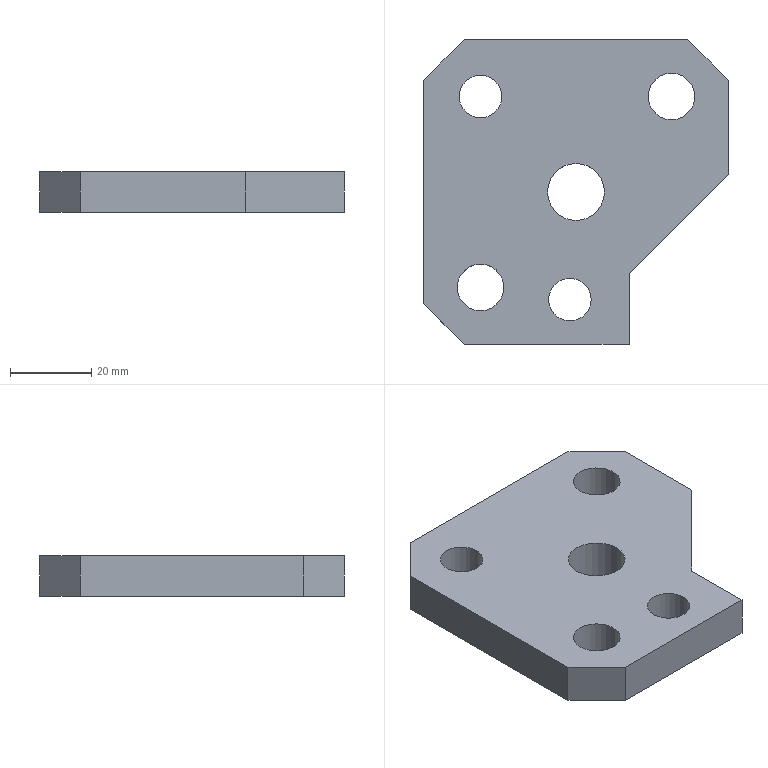Part | NX | features 23 2 | 1 solid | 16 faces | box 75 x 75 x 10 mm | volume 42165 mm3 | plane 11 | cylinder 5 | commonest cylinder face diameters 10.5 x2 11.509 x2 14 x1
STEP:
#1=CARTESIAN_POINT('',(80.279,385.45,-43.5));
#2=VERTEX_POINT('',#1);
#3=CARTESIAN_POINT('',(85.529,385.45,-43.5));
#4=DIRECTION('',(0.,0.,-1.));
#5=DIRECTION('',(-1.,0.,0.));
#6=AXIS2_PLACEMENT_3D('',#3,#4,#5);
#7=CIRCLE('',#6,5.25);
#8=EDGE_CURVE('',#2,#2,#7,.T.);
#9=ORIENTED_EDGE('',*,*,#8,.T.);
#10=EDGE_LOOP('',(#9));
#11=FACE_BOUND('',#10,.T.);
#12=CARTESIAN_POINT('',(80.279,385.45,-33.5));
#13=VERTEX_POINT('',#12);
#14=CARTESIAN_POINT('',(85.529,385.45,-33.5));
#15=DIRECTION('',(0.,0.,-1.));
#16=DIRECTION('',(-1.,0.,0.));
#17=AXIS2_PLACEMENT_3D('',#14,#15,#16);
#18=CIRCLE('',#17,5.25);
#19=EDGE_CURVE('',#13,#13,#18,.T.);
#20=ORIENTED_EDGE('',*,*,#19,.F.);
#21=EDGE_LOOP('',(#20));
#22=FACE_BOUND('',#21,.T.);
#23=CARTESIAN_POINT('',(85.529,385.45,-33.5));
#24=DIRECTION('',(0.,0.,-1.));
#25=DIRECTION('',(0.,-1.,0.));
#26=AXIS2_PLACEMENT_3D('',#23,#24,#25);
#27=CYLINDRICAL_SURFACE('',#26,5.25);
#28=ADVANCED_FACE('',(#11,#22),#27,.F.);
#29=CARTESIAN_POINT('',(80.029,411.95,-33.5));
#30=VERTEX_POINT('',#29);
#31=CARTESIAN_POINT('',(87.029,411.95,-33.5));
#32=DIRECTION('',(0.,0.,1.));
#33=DIRECTION('',(-1.,0.,0.));
#34=AXIS2_PLACEMENT_3D('',#31,#32,#33);
#35=CIRCLE('',#34,7.);
#36=EDGE_CURVE('',#30,#30,#35,.T.);
#37=ORIENTED_EDGE('',*,*,#36,.T.);
#38=EDGE_LOOP('',(#37));
#39=FACE_BOUND('',#38,.T.);
#40=CARTESIAN_POINT('',(80.029,411.95,-43.5));
#41=VERTEX_POINT('',#40);
#42=CARTESIAN_POINT('',(87.029,411.95,-43.5));
#43=DIRECTION('',(0.,0.,1.));
#44=DIRECTION('',(-1.,0.,0.));
#45=AXIS2_PLACEMENT_3D('',#42,#43,#44);
#46=CIRCLE('',#45,7.);
#47=EDGE_CURVE('',#41,#41,#46,.T.);
#48=ORIENTED_EDGE('',*,*,#47,.F.);
#49=EDGE_LOOP('',(#48));
#50=FACE_BOUND('',#49,.T.);
#51=CARTESIAN_POINT('',(87.029,411.95,-33.5));
#52=DIRECTION('',(0.,0.,1.));
#53=DIRECTION('',(0.,1.,0.));
#54=AXIS2_PLACEMENT_3D('',#51,#52,#53);
#55=CYLINDRICAL_SURFACE('',#54,7.);
#56=ADVANCED_FACE('',(#39,#50),#55,.F.);
#57=CARTESIAN_POINT('',(49.529,384.45,-33.5));
#58=VERTEX_POINT('',#57);
#59=CARTESIAN_POINT('',(59.529,374.45,-33.5));
#60=VERTEX_POINT('',#59);
#61=CARTESIAN_POINT('',(55.537,378.441,-33.5));
#62=DIRECTION('',(0.7071,-0.7071,0.));
#63=VECTOR('',#62,1000.);
#64=LINE('',#61,#63);
#65=EDGE_CURVE('',#58,#60,#64,.T.);
#66=ORIENTED_EDGE('',*,*,#65,.F.);
#67=CARTESIAN_POINT('',(49.529,384.45,-43.5));
#68=VERTEX_POINT('',#67);
#69=CARTESIAN_POINT('',(49.529,384.45,-33.5));
#70=DIRECTION('',(0.,0.,1.));
#71=VECTOR('',#70,1000.);
#72=LINE('',#69,#71);
#73=EDGE_CURVE('',#68,#58,#72,.T.);
#74=ORIENTED_EDGE('',*,*,#73,.F.);
#75=CARTESIAN_POINT('',(59.529,374.45,-43.5));
#76=VERTEX_POINT('',#75);
#77=CARTESIAN_POINT('',(54.529,379.45,-43.5));
#78=DIRECTION('',(-0.7071,0.7071,0.));
#79=VECTOR('',#78,1000.);
#80=LINE('',#77,#79);
#81=EDGE_CURVE('',#76,#68,#80,.T.);
#82=ORIENTED_EDGE('',*,*,#81,.F.);
#83=CARTESIAN_POINT('',(59.529,374.45,-33.5));
#84=DIRECTION('',(0.,0.,-1.));
#85=VECTOR('',#84,1000.);
#86=LINE('',#83,#85);
#87=EDGE_CURVE('',#60,#76,#86,.T.);
#88=ORIENTED_EDGE('',*,*,#87,.F.);
#89=EDGE_LOOP('',(#66,#74,#82,#88));
#90=FACE_BOUND('',#89,.T.);
#91=CARTESIAN_POINT('',(54.529,379.45,-23.5));
#92=DIRECTION('',(0.7071,0.7071,0.));
#93=DIRECTION('',(0.,0.,1.));
#94=AXIS2_PLACEMENT_3D('',#91,#92,#93);
#95=PLANE('',#94);
#96=ADVANCED_FACE('',(#90),#95,.F.);
#97=CARTESIAN_POINT('',(49.529,439.45,-33.5));
#98=VERTEX_POINT('',#97);
#99=CARTESIAN_POINT('',(49.529,411.95,-33.5));
#100=DIRECTION('',(0.,-1.,0.));
#101=VECTOR('',#100,1000.);
#102=LINE('',#99,#101);
#103=EDGE_CURVE('',#98,#58,#102,.T.);
#104=ORIENTED_EDGE('',*,*,#103,.F.);
#105=CARTESIAN_POINT('',(49.529,439.45,-43.5));
#106=VERTEX_POINT('',#105);
#107=CARTESIAN_POINT('',(49.529,439.45,-33.5));
#108=DIRECTION('',(0.,0.,-1.));
#109=VECTOR('',#108,1000.);
#110=LINE('',#107,#109);
#111=EDGE_CURVE('',#98,#106,#110,.T.);
#112=ORIENTED_EDGE('',*,*,#111,.T.);
#113=CARTESIAN_POINT('',(49.529,444.376,-43.5));
#114=DIRECTION('',(0.,-1.,0.));
#115=VECTOR('',#114,1000.);
#116=LINE('',#113,#115);
#117=EDGE_CURVE('',#106,#68,#116,.T.);
#118=ORIENTED_EDGE('',*,*,#117,.T.);
#119=ORIENTED_EDGE('',*,*,#73,.T.);
#120=EDGE_LOOP('',(#104,#112,#118,#119));
#121=FACE_BOUND('',#120,.T.);
#122=CARTESIAN_POINT('',(49.529,411.95,-33.5));
#123=DIRECTION('',(1.,0.,0.));
#124=DIRECTION('',(0.,-1.,0.));
#125=AXIS2_PLACEMENT_3D('',#122,#123,#124);
#126=PLANE('',#125);
#127=ADVANCED_FACE('',(#121),#126,.F.);
#128=CARTESIAN_POINT('',(59.529,449.45,-33.5));
#129=VERTEX_POINT('',#128);
#130=CARTESIAN_POINT('',(87.964,477.885,-33.5));
#131=DIRECTION('',(-0.7071,-0.7071,0.));
#132=VECTOR('',#131,1000.);
#133=LINE('',#130,#132);
#134=EDGE_CURVE('',#129,#98,#133,.T.);
#135=ORIENTED_EDGE('',*,*,#134,.F.);
#136=CARTESIAN_POINT('',(59.529,449.45,-43.5));
#137=VERTEX_POINT('',#136);
#138=CARTESIAN_POINT('',(59.529,449.45,-33.5));
#139=DIRECTION('',(0.,0.,1.));
#140=VECTOR('',#139,1000.);
#141=LINE('',#138,#140);
#142=EDGE_CURVE('',#137,#129,#141,.T.);
#143=ORIENTED_EDGE('',*,*,#142,.F.);
#144=CARTESIAN_POINT('',(54.529,444.45,-43.5));
#145=DIRECTION('',(0.7071,0.7071,0.));
#146=VECTOR('',#145,1000.);
#147=LINE('',#144,#146);
#148=EDGE_CURVE('',#106,#137,#147,.T.);
#149=ORIENTED_EDGE('',*,*,#148,.F.);
#150=ORIENTED_EDGE('',*,*,#111,.F.);
#151=EDGE_LOOP('',(#135,#143,#149,#150));
#152=FACE_BOUND('',#151,.T.);
#153=CARTESIAN_POINT('',(54.529,444.45,-23.5));
#154=DIRECTION('',(0.7071,-0.7071,0.));
#155=DIRECTION('',(0.,0.,1.));
#156=AXIS2_PLACEMENT_3D('',#153,#154,#155);
#157=PLANE('',#156);
#158=ADVANCED_FACE('',(#152),#157,.F.);
#159=CARTESIAN_POINT('',(114.529,449.45,-33.5));
#160=VERTEX_POINT('',#159);
#161=CARTESIAN_POINT('',(87.029,449.45,-33.5));
#162=DIRECTION('',(-1.,0.,0.));
#163=VECTOR('',#162,1000.);
#164=LINE('',#161,#163);
#165=EDGE_CURVE('',#160,#129,#164,.T.);
#166=ORIENTED_EDGE('',*,*,#165,.F.);
#167=CARTESIAN_POINT('',(114.529,449.45,-43.5));
#168=VERTEX_POINT('',#167);
#169=CARTESIAN_POINT('',(114.529,449.45,-33.5));
#170=DIRECTION('',(0.,0.,-1.));
#171=VECTOR('',#170,1000.);
#172=LINE('',#169,#171);
#173=EDGE_CURVE('',#160,#168,#172,.T.);
#174=ORIENTED_EDGE('',*,*,#173,.T.);
#175=CARTESIAN_POINT('',(121.472,449.45,-43.5));
#176=DIRECTION('',(-1.,0.,0.));
#177=VECTOR('',#176,1000.);
#178=LINE('',#175,#177);
#179=EDGE_CURVE('',#168,#137,#178,.T.);
#180=ORIENTED_EDGE('',*,*,#179,.T.);
#181=ORIENTED_EDGE('',*,*,#142,.T.);
#182=EDGE_LOOP('',(#166,#174,#180,#181));
#183=FACE_BOUND('',#182,.T.);
#184=CARTESIAN_POINT('',(87.029,449.45,-33.5));
#185=DIRECTION('',(0.,-1.,0.));
#186=DIRECTION('',(-1.,0.,0.));
#187=AXIS2_PLACEMENT_3D('',#184,#185,#186);
#188=PLANE('',#187);
#189=ADVANCED_FACE('',(#183),#188,.F.);
#190=CARTESIAN_POINT('',(124.529,439.45,-33.5));
#191=VERTEX_POINT('',#190);
#192=CARTESIAN_POINT('',(120.537,443.441,-33.5));
#193=DIRECTION('',(-0.7071,0.7071,0.));
#194=VECTOR('',#193,1000.);
#195=LINE('',#192,#194);
#196=EDGE_CURVE('',#191,#160,#195,.T.);
#197=ORIENTED_EDGE('',*,*,#196,.F.);
#198=CARTESIAN_POINT('',(124.529,439.45,-43.5));
#199=VERTEX_POINT('',#198);
#200=CARTESIAN_POINT('',(124.529,439.45,-33.5));
#201=DIRECTION('',(0.,0.,1.));
#202=VECTOR('',#201,1000.);
#203=LINE('',#200,#202);
#204=EDGE_CURVE('',#199,#191,#203,.T.);
#205=ORIENTED_EDGE('',*,*,#204,.F.);
#206=CARTESIAN_POINT('',(124.529,439.45,-43.5));
#207=DIRECTION('',(0.7071,-0.7071,0.));
#208=VECTOR('',#207,1000.);
#209=LINE('',#206,#208);
#210=EDGE_CURVE('',#168,#199,#209,.T.);
#211=ORIENTED_EDGE('',*,*,#210,.F.);
#212=ORIENTED_EDGE('',*,*,#173,.F.);
#213=EDGE_LOOP('',(#197,#205,#211,#212));
#214=FACE_BOUND('',#213,.T.);
#215=CARTESIAN_POINT('',(124.529,439.45,-23.5));
#216=DIRECTION('',(-0.7071,-0.7071,0.));
#217=DIRECTION('',(0.,0.,1.));
#218=AXIS2_PLACEMENT_3D('',#215,#216,#217);
#219=PLANE('',#218);
#220=ADVANCED_FACE('',(#214),#219,.F.);
#221=CARTESIAN_POINT('',(124.529,416.278,-43.5));
#222=VERTEX_POINT('',#221);
#223=CARTESIAN_POINT('',(124.529,444.376,-43.5));
#224=DIRECTION('',(0.,1.,0.));
#225=VECTOR('',#224,1000.);
#226=LINE('',#223,#225);
#227=EDGE_CURVE('',#222,#199,#226,.T.);
#228=ORIENTED_EDGE('',*,*,#227,.T.);
#229=ORIENTED_EDGE('',*,*,#204,.T.);
#230=CARTESIAN_POINT('',(124.529,416.278,-33.5));
#231=VERTEX_POINT('',#230);
#232=CARTESIAN_POINT('',(124.529,411.95,-33.5));
#233=DIRECTION('',(0.,1.,0.));
#234=VECTOR('',#233,1000.);
#235=LINE('',#232,#234);
#236=EDGE_CURVE('',#231,#191,#235,.T.);
#237=ORIENTED_EDGE('',*,*,#236,.F.);
#238=CARTESIAN_POINT('',(124.529,416.278,-33.5));
#239=DIRECTION('',(0.,0.,-1.));
#240=VECTOR('',#239,1000.);
#241=LINE('',#238,#240);
#242=EDGE_CURVE('',#231,#222,#241,.T.);
#243=ORIENTED_EDGE('',*,*,#242,.T.);
#244=EDGE_LOOP('',(#228,#229,#237,#243));
#245=FACE_BOUND('',#244,.T.);
#246=CARTESIAN_POINT('',(124.529,411.95,-33.5));
#247=DIRECTION('',(-1.,0.,0.));
#248=DIRECTION('',(0.,1.,0.));
#249=AXIS2_PLACEMENT_3D('',#246,#247,#248);
#250=PLANE('',#249);
#251=ADVANCED_FACE('',(#245),#250,.F.);
#252=CARTESIAN_POINT('',(100.109,391.859,-33.5));
#253=VERTEX_POINT('',#252);
#254=CARTESIAN_POINT('',(137.049,428.799,-33.5));
#255=DIRECTION('',(0.7071,0.7071,0.));
#256=VECTOR('',#255,1000.);
#257=LINE('',#254,#256);
#258=EDGE_CURVE('',#253,#231,#257,.T.);
#259=ORIENTED_EDGE('',*,*,#258,.F.);
#260=CARTESIAN_POINT('',(100.109,391.859,-43.5));
#261=VERTEX_POINT('',#260);
#262=CARTESIAN_POINT('',(100.109,391.859,-33.5));
#263=DIRECTION('',(0.,0.,-1.));
#264=VECTOR('',#263,1000.);
#265=LINE('',#262,#264);
#266=EDGE_CURVE('',#253,#261,#265,.T.);
#267=ORIENTED_EDGE('',*,*,#266,.T.);
#268=CARTESIAN_POINT('',(123.114,414.864,-43.5));
#269=DIRECTION('',(-0.7071,-0.7071,0.));
#270=VECTOR('',#269,1000.);
#271=LINE('',#268,#270);
#272=EDGE_CURVE('',#222,#261,#271,.T.);
#273=ORIENTED_EDGE('',*,*,#272,.F.);
#274=ORIENTED_EDGE('',*,*,#242,.F.);
#275=EDGE_LOOP('',(#259,#267,#273,#274));
#276=FACE_BOUND('',#275,.T.);
#277=CARTESIAN_POINT('',(123.114,414.864,-33.5));
#278=DIRECTION('',(-0.7071,0.7071,0.));
#279=DIRECTION('',(0.,0.,-1.));
#280=AXIS2_PLACEMENT_3D('',#277,#278,#279);
#281=PLANE('',#280);
#282=ADVANCED_FACE('',(#276),#281,.F.);
#283=CARTESIAN_POINT('',(100.109,374.45,-43.5));
#284=VERTEX_POINT('',#283);
#285=CARTESIAN_POINT('',(100.109,444.376,-43.5));
#286=DIRECTION('',(0.,-1.,0.));
#287=VECTOR('',#286,1000.);
#288=LINE('',#285,#287);
#289=EDGE_CURVE('',#261,#284,#288,.T.);
#290=ORIENTED_EDGE('',*,*,#289,.F.);
#291=ORIENTED_EDGE('',*,*,#266,.F.);
#292=CARTESIAN_POINT('',(100.109,374.45,-33.5));
#293=VERTEX_POINT('',#292);
#294=CARTESIAN_POINT('',(100.109,392.723,-33.5));
#295=DIRECTION('',(0.,1.,0.));
#296=VECTOR('',#295,1000.);
#297=LINE('',#294,#296);
#298=EDGE_CURVE('',#293,#253,#297,.T.);
#299=ORIENTED_EDGE('',*,*,#298,.F.);
#300=CARTESIAN_POINT('',(100.109,374.45,-8.5));
#301=DIRECTION('',(0.,0.,1.));
#302=VECTOR('',#301,1000.);
#303=LINE('',#300,#302);
#304=EDGE_CURVE('',#284,#293,#303,.T.);
#305=ORIENTED_EDGE('',*,*,#304,.F.);
#306=EDGE_LOOP('',(#290,#291,#299,#305));
#307=FACE_BOUND('',#306,.T.);
#308=CARTESIAN_POINT('',(100.109,392.723,-8.5));
#309=DIRECTION('',(-1.,0.,0.));
#310=DIRECTION('',(0.,0.,1.));
#311=AXIS2_PLACEMENT_3D('',#308,#309,#310);
#312=PLANE('',#311);
#313=ADVANCED_FACE('',(#307),#312,.F.);
#314=CARTESIAN_POINT('',(121.472,374.45,-43.5));
#315=DIRECTION('',(1.,0.,0.));
#316=VECTOR('',#315,1000.);
#317=LINE('',#314,#316);
#318=EDGE_CURVE('',#76,#284,#317,.T.);
#319=ORIENTED_EDGE('',*,*,#318,.T.);
#320=ORIENTED_EDGE('',*,*,#304,.T.);
#321=CARTESIAN_POINT('',(87.029,374.45,-33.5));
#322=DIRECTION('',(1.,0.,0.));
#323=VECTOR('',#322,1000.);
#324=LINE('',#321,#323);
#325=EDGE_CURVE('',#60,#293,#324,.T.);
#326=ORIENTED_EDGE('',*,*,#325,.F.);
#327=ORIENTED_EDGE('',*,*,#87,.T.);
#328=EDGE_LOOP('',(#319,#320,#326,#327));
#329=FACE_BOUND('',#328,.T.);
#330=CARTESIAN_POINT('',(87.029,374.45,-33.5));
#331=DIRECTION('',(0.,1.,0.));
#332=DIRECTION('',(1.,0.,0.));
#333=AXIS2_PLACEMENT_3D('',#330,#331,#332);
#334=PLANE('',#333);
#335=ADVANCED_FACE('',(#329),#334,.F.);
#336=CARTESIAN_POINT('',(110.529,429.695,-43.5));
#337=VERTEX_POINT('',#336);
#338=CARTESIAN_POINT('',(110.529,435.45,-43.5));
#339=DIRECTION('',(0.,0.,-1.));
#340=DIRECTION('',(0.,-1.,0.));
#341=AXIS2_PLACEMENT_3D('',#338,#339,#340);
#342=CIRCLE('',#341,5.755);
#343=EDGE_CURVE('',#337,#337,#342,.T.);
#344=ORIENTED_EDGE('',*,*,#343,.T.);
#345=EDGE_LOOP('',(#344));
#346=FACE_BOUND('',#345,.T.);
#347=CARTESIAN_POINT('',(110.529,429.695,-33.5));
#348=VERTEX_POINT('',#347);
#349=CARTESIAN_POINT('',(110.529,435.45,-33.5));
#350=DIRECTION('',(0.,0.,-1.));
#351=DIRECTION('',(0.,-1.,0.));
#352=AXIS2_PLACEMENT_3D('',#349,#350,#351);
#353=CIRCLE('',#352,5.755);
#354=EDGE_CURVE('',#348,#348,#353,.T.);
#355=ORIENTED_EDGE('',*,*,#354,.F.);
#356=EDGE_LOOP('',(#355));
#357=FACE_BOUND('',#356,.T.);
#358=CARTESIAN_POINT('',(110.529,435.45,-33.5));
#359=DIRECTION('',(0.,0.,-1.));
#360=DIRECTION('',(0.,-1.,0.));
#361=AXIS2_PLACEMENT_3D('',#358,#359,#360);
#362=CYLINDRICAL_SURFACE('',#361,5.755);
#363=ADVANCED_FACE('',(#346,#357),#362,.F.);
#364=CARTESIAN_POINT('',(63.529,430.2,-43.5));
#365=VERTEX_POINT('',#364);
#366=CARTESIAN_POINT('',(63.529,435.45,-43.5));
#367=DIRECTION('',(0.,0.,-1.));
#368=DIRECTION('',(0.,-1.,0.));
#369=AXIS2_PLACEMENT_3D('',#366,#367,#368);
#370=CIRCLE('',#369,5.25);
#371=EDGE_CURVE('',#365,#365,#370,.T.);
#372=ORIENTED_EDGE('',*,*,#371,.T.);
#373=EDGE_LOOP('',(#372));
#374=FACE_BOUND('',#373,.T.);
#375=CARTESIAN_POINT('',(63.529,430.2,-33.5));
#376=VERTEX_POINT('',#375);
#377=CARTESIAN_POINT('',(63.529,435.45,-33.5));
#378=DIRECTION('',(0.,0.,-1.));
#379=DIRECTION('',(0.,-1.,0.));
#380=AXIS2_PLACEMENT_3D('',#377,#378,#379);
#381=CIRCLE('',#380,5.25);
#382=EDGE_CURVE('',#376,#376,#381,.T.);
#383=ORIENTED_EDGE('',*,*,#382,.F.);
#384=EDGE_LOOP('',(#383));
#385=FACE_BOUND('',#384,.T.);
#386=CARTESIAN_POINT('',(63.529,435.45,-33.5));
#387=DIRECTION('',(0.,0.,-1.));
#388=DIRECTION('',(0.,-1.,0.));
#389=AXIS2_PLACEMENT_3D('',#386,#387,#388);
#390=CYLINDRICAL_SURFACE('',#389,5.25);
#391=ADVANCED_FACE('',(#374,#385),#390,.F.);
#392=CARTESIAN_POINT('',(63.529,382.695,-43.5));
#393=VERTEX_POINT('',#392);
#394=CARTESIAN_POINT('',(63.529,388.45,-43.5));
#395=DIRECTION('',(0.,0.,-1.));
#396=DIRECTION('',(0.,-1.,0.));
#397=AXIS2_PLACEMENT_3D('',#394,#395,#396);
#398=CIRCLE('',#397,5.755);
#399=EDGE_CURVE('',#393,#393,#398,.T.);
#400=ORIENTED_EDGE('',*,*,#399,.T.);
#401=EDGE_LOOP('',(#400));
#402=FACE_BOUND('',#401,.T.);
#403=CARTESIAN_POINT('',(63.529,382.695,-33.5));
#404=VERTEX_POINT('',#403);
#405=CARTESIAN_POINT('',(63.529,388.45,-33.5));
#406=DIRECTION('',(0.,0.,-1.));
#407=DIRECTION('',(0.,-1.,0.));
#408=AXIS2_PLACEMENT_3D('',#405,#406,#407);
#409=CIRCLE('',#408,5.755);
#410=EDGE_CURVE('',#404,#404,#409,.T.);
#411=ORIENTED_EDGE('',*,*,#410,.F.);
#412=EDGE_LOOP('',(#411));
#413=FACE_BOUND('',#412,.T.);
#414=CARTESIAN_POINT('',(63.529,388.45,-33.5));
#415=DIRECTION('',(0.,0.,-1.));
#416=DIRECTION('',(0.,-1.,0.));
#417=AXIS2_PLACEMENT_3D('',#414,#415,#416);
#418=CYLINDRICAL_SURFACE('',#417,5.755);
#419=ADVANCED_FACE('',(#402,#413),#418,.F.);
#420=ORIENTED_EDGE('',*,*,#19,.T.);
#421=EDGE_LOOP('',(#420));
#422=FACE_BOUND('',#421,.T.);
#423=ORIENTED_EDGE('',*,*,#410,.T.);
#424=EDGE_LOOP('',(#423));
#425=FACE_BOUND('',#424,.T.);
#426=ORIENTED_EDGE('',*,*,#382,.T.);
#427=EDGE_LOOP('',(#426));
#428=FACE_BOUND('',#427,.T.);
#429=ORIENTED_EDGE('',*,*,#354,.T.);
#430=EDGE_LOOP('',(#429));
#431=FACE_BOUND('',#430,.T.);
#432=ORIENTED_EDGE('',*,*,#325,.T.);
#433=ORIENTED_EDGE('',*,*,#298,.T.);
#434=ORIENTED_EDGE('',*,*,#258,.T.);
#435=ORIENTED_EDGE('',*,*,#236,.T.);
#436=ORIENTED_EDGE('',*,*,#196,.T.);
#437=ORIENTED_EDGE('',*,*,#165,.T.);
#438=ORIENTED_EDGE('',*,*,#134,.T.);
#439=ORIENTED_EDGE('',*,*,#103,.T.);
#440=ORIENTED_EDGE('',*,*,#65,.T.);
#441=EDGE_LOOP('',(#432,#433,#434,#435,#436,#437,#438,#439,#440));
#442=FACE_BOUND('',#441,.T.);
#443=ORIENTED_EDGE('',*,*,#36,.F.);
#444=EDGE_LOOP('',(#443));
#445=FACE_BOUND('',#444,.T.);
#446=CARTESIAN_POINT('',(121.472,444.376,-33.5));
#447=DIRECTION('',(0.,0.,-1.));
#448=DIRECTION('',(0.,-1.,0.));
#449=AXIS2_PLACEMENT_3D('',#446,#447,#448);
#450=PLANE('',#449);
#451=ADVANCED_FACE('',(#422,#425,#428,#431,#442,#445),#450,.F.);
#452=ORIENTED_EDGE('',*,*,#8,.F.);
#453=EDGE_LOOP('',(#452));
#454=FACE_BOUND('',#453,.T.);
#455=ORIENTED_EDGE('',*,*,#399,.F.);
#456=EDGE_LOOP('',(#455));
#457=FACE_BOUND('',#456,.T.);
#458=ORIENTED_EDGE('',*,*,#371,.F.);
#459=EDGE_LOOP('',(#458));
#460=FACE_BOUND('',#459,.T.);
#461=ORIENTED_EDGE('',*,*,#343,.F.);
#462=EDGE_LOOP('',(#461));
#463=FACE_BOUND('',#462,.T.);
#464=ORIENTED_EDGE('',*,*,#272,.T.);
#465=ORIENTED_EDGE('',*,*,#289,.T.);
#466=ORIENTED_EDGE('',*,*,#318,.F.);
#467=ORIENTED_EDGE('',*,*,#81,.T.);
#468=ORIENTED_EDGE('',*,*,#117,.F.);
#469=ORIENTED_EDGE('',*,*,#148,.T.);
#470=ORIENTED_EDGE('',*,*,#179,.F.);
#471=ORIENTED_EDGE('',*,*,#210,.T.);
#472=ORIENTED_EDGE('',*,*,#227,.F.);
#473=EDGE_LOOP('',(#464,#465,#466,#467,#468,#469,#470,#471,#472));
#474=FACE_BOUND('',#473,.T.);
#475=ORIENTED_EDGE('',*,*,#47,.T.);
#476=EDGE_LOOP('',(#475));
#477=FACE_BOUND('',#476,.T.);
#478=CARTESIAN_POINT('',(121.472,444.376,-43.5));
#479=DIRECTION('',(0.,0.,-1.));
#480=DIRECTION('',(0.,-1.,0.));
#481=AXIS2_PLACEMENT_3D('',#478,#479,#480);
#482=PLANE('',#481);
#483=ADVANCED_FACE('',(#454,#457,#460,#463,#474,#477),#482,.T.);
#484=CLOSED_SHELL('',(#28,#56,#96,#127,#158,#189,#220,#251,#282,#313,#335,#363,#391,#419,#451,#483));
#485=MANIFOLD_SOLID_BREP('',#484);
#486=(LENGTH_UNIT()NAMED_UNIT(*)SI_UNIT(.MILLI.,.METRE.));
#487=UNCERTAINTY_MEASURE_WITH_UNIT(LENGTH_MEASURE(0.00001),#486,'','');
#488=(NAMED_UNIT(*)PLANE_ANGLE_UNIT()SI_UNIT($,.RADIAN.));
#489=(NAMED_UNIT(*)SI_UNIT($,.STERADIAN.)SOLID_ANGLE_UNIT());
#490=(GEOMETRIC_REPRESENTATION_CONTEXT(3)GLOBAL_UNCERTAINTY_ASSIGNED_CONTEXT((#487))GLOBAL_UNIT_ASSIGNED_CONTEXT((#486,#488,#489))REPRESENTATION_CONTEXT('',''));
#491=ADVANCED_BREP_SHAPE_REPRESENTATION('',(#485),#490);